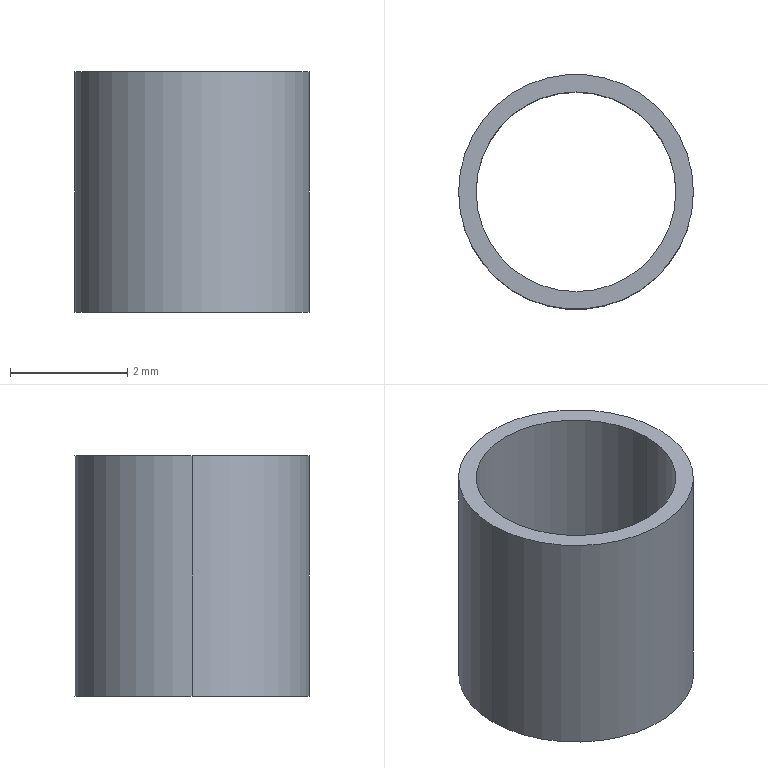Part | STEP file | Height-limit steel tube | 1 solid | 6 faces | box 4 x 4 x 4.1 mm | volume 14.297 mm3 | cylinder 4 | plane 2 | commonest cylinder face diameters 3.4 x2 4 x2
STEP:
#1=CARTESIAN_POINT('',(0.,0.,0.));
#2=DIRECTION('',(0.,0.,1.));
#3=DIRECTION('',(1.,0.,0.));
#4=AXIS2_PLACEMENT_3D('',#1,#2,#3);
#5=CARTESIAN_POINT('',(-1.7,0.,4.1));
#6=VERTEX_POINT('',#5);
#7=CARTESIAN_POINT('',(-1.7,0.,0.));
#8=VERTEX_POINT('',#7);
#9=CARTESIAN_POINT('',(-1.7,0.,4.1));
#10=DIRECTION('',(0.,0.,-1.));
#11=VECTOR('',#10,1.);
#12=LINE('',#9,#11);
#13=CARTESIAN_POINT('',(0.,0.,4.1));
#14=DIRECTION('',(0.,0.,-1.));
#15=DIRECTION('',(-1.,0.,0.));
#16=AXIS2_PLACEMENT_3D('',#13,#14,#15);
#17=CYLINDRICAL_SURFACE('',#16,1.7);
#18=CARTESIAN_POINT('',(6.283,0.));
#19=DIRECTION('',(0.,1.));
#20=VECTOR('',#19,1.);
#21=LINE('',#18,#20);
#22=(GEOMETRIC_REPRESENTATION_CONTEXT(2)PARAMETRIC_REPRESENTATION_CONTEXT()REPRESENTATION_CONTEXT('',''));
#23=DEFINITIONAL_REPRESENTATION('',(#21),#22);
#24=PCURVE('',#17,#23);
#25=CARTESIAN_POINT('',(0.,0.,4.1));
#26=DIRECTION('',(0.,0.,-1.));
#27=DIRECTION('',(-1.,0.,0.));
#28=AXIS2_PLACEMENT_3D('',#25,#26,#27);
#29=CYLINDRICAL_SURFACE('',#28,1.7);
#30=CARTESIAN_POINT('',(0.,0.));
#31=DIRECTION('',(0.,1.));
#32=VECTOR('',#31,1.);
#33=LINE('',#30,#32);
#34=(GEOMETRIC_REPRESENTATION_CONTEXT(2)PARAMETRIC_REPRESENTATION_CONTEXT()REPRESENTATION_CONTEXT('',''));
#35=DEFINITIONAL_REPRESENTATION('',(#33),#34);
#36=PCURVE('',#29,#35);
#37=SURFACE_CURVE('',#12,(#24,#36),.PCURVE_S1.);
#38=EDGE_CURVE('',#6,#8,#37,.T.);
#39=ORIENTED_EDGE('',*,*,#38,.T.);
#40=CARTESIAN_POINT('',(1.7,0.,0.));
#41=VERTEX_POINT('',#40);
#42=CARTESIAN_POINT('',(0.,0.,0.));
#43=DIRECTION('',(0.,0.,1.));
#44=DIRECTION('',(1.,0.,0.));
#45=AXIS2_PLACEMENT_3D('',#42,#43,#44);
#46=CIRCLE('',#45,1.7);
#47=CARTESIAN_POINT('',(9.425,4.1));
#48=DIRECTION('',(-1.,0.));
#49=VECTOR('',#48,1.);
#50=LINE('',#47,#49);
#51=(GEOMETRIC_REPRESENTATION_CONTEXT(2)PARAMETRIC_REPRESENTATION_CONTEXT()REPRESENTATION_CONTEXT('',''));
#52=DEFINITIONAL_REPRESENTATION('',(#50),#51);
#53=PCURVE('',#17,#52);
#54=CARTESIAN_POINT('',(0.,0.,0.));
#55=DIRECTION('',(0.,0.,1.));
#56=DIRECTION('',(1.,0.,0.));
#57=AXIS2_PLACEMENT_3D('',#54,#55,#56);
#58=PLANE('',#57);
#59=CARTESIAN_POINT('',(0.,0.));
#60=DIRECTION('',(1.,0.));
#61=AXIS2_PLACEMENT_2D('',#59,#60);
#62=CIRCLE('',#61,1.7);
#63=(GEOMETRIC_REPRESENTATION_CONTEXT(2)PARAMETRIC_REPRESENTATION_CONTEXT()REPRESENTATION_CONTEXT('',''));
#64=DEFINITIONAL_REPRESENTATION('',(#62),#63);
#65=PCURVE('',#58,#64);
#66=SURFACE_CURVE('',#46,(#53,#65),.PCURVE_S1.);
#67=EDGE_CURVE('',#8,#41,#66,.T.);
#68=ORIENTED_EDGE('',*,*,#67,.T.);
#69=CARTESIAN_POINT('',(1.7,0.,4.1));
#70=VERTEX_POINT('',#69);
#71=CARTESIAN_POINT('',(1.7,0.,4.1));
#72=DIRECTION('',(0.,0.,-1.));
#73=VECTOR('',#72,1.);
#74=LINE('',#71,#73);
#75=CARTESIAN_POINT('',(3.142,0.));
#76=DIRECTION('',(0.,1.));
#77=VECTOR('',#76,1.);
#78=LINE('',#75,#77);
#79=(GEOMETRIC_REPRESENTATION_CONTEXT(2)PARAMETRIC_REPRESENTATION_CONTEXT()REPRESENTATION_CONTEXT('',''));
#80=DEFINITIONAL_REPRESENTATION('',(#78),#79);
#81=PCURVE('',#17,#80);
#82=CARTESIAN_POINT('',(3.142,0.));
#83=DIRECTION('',(0.,1.));
#84=VECTOR('',#83,1.);
#85=LINE('',#82,#84);
#86=(GEOMETRIC_REPRESENTATION_CONTEXT(2)PARAMETRIC_REPRESENTATION_CONTEXT()REPRESENTATION_CONTEXT('',''));
#87=DEFINITIONAL_REPRESENTATION('',(#85),#86);
#88=PCURVE('',#29,#87);
#89=SURFACE_CURVE('',#74,(#81,#88),.PCURVE_S1.);
#90=EDGE_CURVE('',#70,#41,#89,.T.);
#91=ORIENTED_EDGE('',*,*,#90,.F.);
#92=CARTESIAN_POINT('',(0.,0.,4.1));
#93=DIRECTION('',(0.,0.,1.));
#94=DIRECTION('',(1.,0.,0.));
#95=AXIS2_PLACEMENT_3D('',#92,#93,#94);
#96=CIRCLE('',#95,1.7);
#97=CARTESIAN_POINT('',(9.425,0.));
#98=DIRECTION('',(-1.,0.));
#99=VECTOR('',#98,1.);
#100=LINE('',#97,#99);
#101=(GEOMETRIC_REPRESENTATION_CONTEXT(2)PARAMETRIC_REPRESENTATION_CONTEXT()REPRESENTATION_CONTEXT('',''));
#102=DEFINITIONAL_REPRESENTATION('',(#100),#101);
#103=PCURVE('',#17,#102);
#104=CARTESIAN_POINT('',(0.,0.,4.1));
#105=DIRECTION('',(0.,0.,1.));
#106=DIRECTION('',(1.,0.,0.));
#107=AXIS2_PLACEMENT_3D('',#104,#105,#106);
#108=PLANE('',#107);
#109=CARTESIAN_POINT('',(0.,0.));
#110=DIRECTION('',(1.,0.));
#111=AXIS2_PLACEMENT_2D('',#109,#110);
#112=CIRCLE('',#111,1.7);
#113=(GEOMETRIC_REPRESENTATION_CONTEXT(2)PARAMETRIC_REPRESENTATION_CONTEXT()REPRESENTATION_CONTEXT('',''));
#114=DEFINITIONAL_REPRESENTATION('',(#112),#113);
#115=PCURVE('',#108,#114);
#116=SURFACE_CURVE('',#96,(#103,#115),.PCURVE_S1.);
#117=EDGE_CURVE('',#6,#70,#116,.T.);
#118=ORIENTED_EDGE('',*,*,#117,.F.);
#119=EDGE_LOOP('',(#39,#68,#91,#118));
#120=FACE_BOUND('',#119,.F.);
#121=ADVANCED_FACE('',(#120),#17,.F.);
#122=CARTESIAN_POINT('',(2.,0.,4.1));
#123=VERTEX_POINT('',#122);
#124=CARTESIAN_POINT('',(-2.,0.,4.1));
#125=VERTEX_POINT('',#124);
#126=CARTESIAN_POINT('',(0.,0.,4.1));
#127=DIRECTION('',(0.,0.,1.));
#128=DIRECTION('',(1.,0.,0.));
#129=AXIS2_PLACEMENT_3D('',#126,#127,#128);
#130=CIRCLE('',#129,2.);
#131=CARTESIAN_POINT('',(0.,0.,4.1));
#132=DIRECTION('',(0.,0.,-1.));
#133=DIRECTION('',(-1.,0.,0.));
#134=AXIS2_PLACEMENT_3D('',#131,#132,#133);
#135=CYLINDRICAL_SURFACE('',#134,2.);
#136=CARTESIAN_POINT('',(3.142,0.));
#137=DIRECTION('',(-1.,0.));
#138=VECTOR('',#137,1.);
#139=LINE('',#136,#138);
#140=(GEOMETRIC_REPRESENTATION_CONTEXT(2)PARAMETRIC_REPRESENTATION_CONTEXT()REPRESENTATION_CONTEXT('',''));
#141=DEFINITIONAL_REPRESENTATION('',(#139),#140);
#142=PCURVE('',#135,#141);
#143=CARTESIAN_POINT('',(0.,0.));
#144=DIRECTION('',(1.,0.));
#145=AXIS2_PLACEMENT_2D('',#143,#144);
#146=CIRCLE('',#145,2.);
#147=(GEOMETRIC_REPRESENTATION_CONTEXT(2)PARAMETRIC_REPRESENTATION_CONTEXT()REPRESENTATION_CONTEXT('',''));
#148=DEFINITIONAL_REPRESENTATION('',(#146),#147);
#149=PCURVE('',#108,#148);
#150=SURFACE_CURVE('',#130,(#142,#149),.PCURVE_S1.);
#151=EDGE_CURVE('',#123,#125,#150,.T.);
#152=ORIENTED_EDGE('',*,*,#151,.F.);
#153=CARTESIAN_POINT('',(2.,0.,0.));
#154=VERTEX_POINT('',#153);
#155=CARTESIAN_POINT('',(2.,0.,4.1));
#156=DIRECTION('',(0.,0.,-1.));
#157=VECTOR('',#156,1.);
#158=LINE('',#155,#157);
#159=CARTESIAN_POINT('',(3.142,0.));
#160=DIRECTION('',(0.,1.));
#161=VECTOR('',#160,1.);
#162=LINE('',#159,#161);
#163=(GEOMETRIC_REPRESENTATION_CONTEXT(2)PARAMETRIC_REPRESENTATION_CONTEXT()REPRESENTATION_CONTEXT('',''));
#164=DEFINITIONAL_REPRESENTATION('',(#162),#163);
#165=PCURVE('',#135,#164);
#166=CARTESIAN_POINT('',(0.,0.,4.1));
#167=DIRECTION('',(0.,0.,-1.));
#168=DIRECTION('',(-1.,0.,0.));
#169=AXIS2_PLACEMENT_3D('',#166,#167,#168);
#170=CYLINDRICAL_SURFACE('',#169,2.);
#171=CARTESIAN_POINT('',(3.142,0.));
#172=DIRECTION('',(0.,1.));
#173=VECTOR('',#172,1.);
#174=LINE('',#171,#173);
#175=(GEOMETRIC_REPRESENTATION_CONTEXT(2)PARAMETRIC_REPRESENTATION_CONTEXT()REPRESENTATION_CONTEXT('',''));
#176=DEFINITIONAL_REPRESENTATION('',(#174),#175);
#177=PCURVE('',#170,#176);
#178=SURFACE_CURVE('',#158,(#165,#177),.PCURVE_S1.);
#179=EDGE_CURVE('',#123,#154,#178,.T.);
#180=ORIENTED_EDGE('',*,*,#179,.T.);
#181=CARTESIAN_POINT('',(-2.,0.,0.));
#182=VERTEX_POINT('',#181);
#183=CARTESIAN_POINT('',(0.,0.,0.));
#184=DIRECTION('',(0.,0.,1.));
#185=DIRECTION('',(1.,0.,0.));
#186=AXIS2_PLACEMENT_3D('',#183,#184,#185);
#187=CIRCLE('',#186,2.);
#188=CARTESIAN_POINT('',(3.142,4.1));
#189=DIRECTION('',(-1.,0.));
#190=VECTOR('',#189,1.);
#191=LINE('',#188,#190);
#192=(GEOMETRIC_REPRESENTATION_CONTEXT(2)PARAMETRIC_REPRESENTATION_CONTEXT()REPRESENTATION_CONTEXT('',''));
#193=DEFINITIONAL_REPRESENTATION('',(#191),#192);
#194=PCURVE('',#135,#193);
#195=CARTESIAN_POINT('',(0.,0.));
#196=DIRECTION('',(1.,0.));
#197=AXIS2_PLACEMENT_2D('',#195,#196);
#198=CIRCLE('',#197,2.);
#199=(GEOMETRIC_REPRESENTATION_CONTEXT(2)PARAMETRIC_REPRESENTATION_CONTEXT()REPRESENTATION_CONTEXT('',''));
#200=DEFINITIONAL_REPRESENTATION('',(#198),#199);
#201=PCURVE('',#58,#200);
#202=SURFACE_CURVE('',#187,(#194,#201),.PCURVE_S1.);
#203=EDGE_CURVE('',#154,#182,#202,.T.);
#204=ORIENTED_EDGE('',*,*,#203,.T.);
#205=CARTESIAN_POINT('',(-2.,0.,4.1));
#206=DIRECTION('',(0.,0.,-1.));
#207=VECTOR('',#206,1.);
#208=LINE('',#205,#207);
#209=CARTESIAN_POINT('',(0.,0.));
#210=DIRECTION('',(0.,1.));
#211=VECTOR('',#210,1.);
#212=LINE('',#209,#211);
#213=(GEOMETRIC_REPRESENTATION_CONTEXT(2)PARAMETRIC_REPRESENTATION_CONTEXT()REPRESENTATION_CONTEXT('',''));
#214=DEFINITIONAL_REPRESENTATION('',(#212),#213);
#215=PCURVE('',#135,#214);
#216=CARTESIAN_POINT('',(6.283,0.));
#217=DIRECTION('',(0.,1.));
#218=VECTOR('',#217,1.);
#219=LINE('',#216,#218);
#220=(GEOMETRIC_REPRESENTATION_CONTEXT(2)PARAMETRIC_REPRESENTATION_CONTEXT()REPRESENTATION_CONTEXT('',''));
#221=DEFINITIONAL_REPRESENTATION('',(#219),#220);
#222=PCURVE('',#170,#221);
#223=SURFACE_CURVE('',#208,(#215,#222),.PCURVE_S1.);
#224=EDGE_CURVE('',#125,#182,#223,.T.);
#225=ORIENTED_EDGE('',*,*,#224,.F.);
#226=EDGE_LOOP('',(#152,#180,#204,#225));
#227=FACE_BOUND('',#226,.T.);
#228=ADVANCED_FACE('',(#227),#135,.T.);
#229=CARTESIAN_POINT('',(0.,0.,4.1));
#230=DIRECTION('',(0.,0.,1.));
#231=DIRECTION('',(1.,0.,0.));
#232=AXIS2_PLACEMENT_3D('',#229,#230,#231);
#233=CIRCLE('',#232,2.);
#234=CARTESIAN_POINT('',(0.,0.));
#235=DIRECTION('',(1.,0.));
#236=AXIS2_PLACEMENT_2D('',#234,#235);
#237=CIRCLE('',#236,2.);
#238=(GEOMETRIC_REPRESENTATION_CONTEXT(2)PARAMETRIC_REPRESENTATION_CONTEXT()REPRESENTATION_CONTEXT('',''));
#239=DEFINITIONAL_REPRESENTATION('',(#237),#238);
#240=PCURVE('',#108,#239);
#241=CARTESIAN_POINT('',(9.425,0.));
#242=DIRECTION('',(-1.,0.));
#243=VECTOR('',#242,1.);
#244=LINE('',#241,#243);
#245=(GEOMETRIC_REPRESENTATION_CONTEXT(2)PARAMETRIC_REPRESENTATION_CONTEXT()REPRESENTATION_CONTEXT('',''));
#246=DEFINITIONAL_REPRESENTATION('',(#244),#245);
#247=PCURVE('',#170,#246);
#248=SURFACE_CURVE('',#233,(#240,#247),.PCURVE_S1.);
#249=EDGE_CURVE('',#125,#123,#248,.T.);
#250=ORIENTED_EDGE('',*,*,#249,.T.);
#251=ORIENTED_EDGE('',*,*,#151,.T.);
#252=EDGE_LOOP('',(#250,#251));
#253=FACE_BOUND('',#252,.T.);
#254=ORIENTED_EDGE('',*,*,#117,.F.);
#255=CARTESIAN_POINT('',(0.,0.,4.1));
#256=DIRECTION('',(0.,0.,1.));
#257=DIRECTION('',(1.,0.,0.));
#258=AXIS2_PLACEMENT_3D('',#255,#256,#257);
#259=CIRCLE('',#258,1.7);
#260=CARTESIAN_POINT('',(0.,0.));
#261=DIRECTION('',(1.,0.));
#262=AXIS2_PLACEMENT_2D('',#260,#261);
#263=CIRCLE('',#262,1.7);
#264=(GEOMETRIC_REPRESENTATION_CONTEXT(2)PARAMETRIC_REPRESENTATION_CONTEXT()REPRESENTATION_CONTEXT('',''));
#265=DEFINITIONAL_REPRESENTATION('',(#263),#264);
#266=PCURVE('',#108,#265);
#267=CARTESIAN_POINT('',(3.142,0.));
#268=DIRECTION('',(-1.,0.));
#269=VECTOR('',#268,1.);
#270=LINE('',#267,#269);
#271=(GEOMETRIC_REPRESENTATION_CONTEXT(2)PARAMETRIC_REPRESENTATION_CONTEXT()REPRESENTATION_CONTEXT('',''));
#272=DEFINITIONAL_REPRESENTATION('',(#270),#271);
#273=PCURVE('',#29,#272);
#274=SURFACE_CURVE('',#259,(#266,#273),.PCURVE_S1.);
#275=EDGE_CURVE('',#70,#6,#274,.T.);
#276=ORIENTED_EDGE('',*,*,#275,.F.);
#277=EDGE_LOOP('',(#254,#276));
#278=FACE_BOUND('',#277,.T.);
#279=ADVANCED_FACE('',(#253,#278),#108,.T.);
#280=CARTESIAN_POINT('',(0.,0.,0.));
#281=DIRECTION('',(0.,0.,1.));
#282=DIRECTION('',(1.,0.,0.));
#283=AXIS2_PLACEMENT_3D('',#280,#281,#282);
#284=CIRCLE('',#283,2.);
#285=CARTESIAN_POINT('',(0.,0.));
#286=DIRECTION('',(1.,0.));
#287=AXIS2_PLACEMENT_2D('',#285,#286);
#288=CIRCLE('',#287,2.);
#289=(GEOMETRIC_REPRESENTATION_CONTEXT(2)PARAMETRIC_REPRESENTATION_CONTEXT()REPRESENTATION_CONTEXT('',''));
#290=DEFINITIONAL_REPRESENTATION('',(#288),#289);
#291=PCURVE('',#58,#290);
#292=CARTESIAN_POINT('',(9.425,4.1));
#293=DIRECTION('',(-1.,0.));
#294=VECTOR('',#293,1.);
#295=LINE('',#292,#294);
#296=(GEOMETRIC_REPRESENTATION_CONTEXT(2)PARAMETRIC_REPRESENTATION_CONTEXT()REPRESENTATION_CONTEXT('',''));
#297=DEFINITIONAL_REPRESENTATION('',(#295),#296);
#298=PCURVE('',#170,#297);
#299=SURFACE_CURVE('',#284,(#291,#298),.PCURVE_S1.);
#300=EDGE_CURVE('',#182,#154,#299,.T.);
#301=ORIENTED_EDGE('',*,*,#300,.F.);
#302=ORIENTED_EDGE('',*,*,#203,.F.);
#303=EDGE_LOOP('',(#301,#302));
#304=FACE_BOUND('',#303,.T.);
#305=ORIENTED_EDGE('',*,*,#67,.T.);
#306=CARTESIAN_POINT('',(0.,0.,0.));
#307=DIRECTION('',(0.,0.,1.));
#308=DIRECTION('',(1.,0.,0.));
#309=AXIS2_PLACEMENT_3D('',#306,#307,#308);
#310=CIRCLE('',#309,1.7);
#311=CARTESIAN_POINT('',(0.,0.));
#312=DIRECTION('',(1.,0.));
#313=AXIS2_PLACEMENT_2D('',#311,#312);
#314=CIRCLE('',#313,1.7);
#315=(GEOMETRIC_REPRESENTATION_CONTEXT(2)PARAMETRIC_REPRESENTATION_CONTEXT()REPRESENTATION_CONTEXT('',''));
#316=DEFINITIONAL_REPRESENTATION('',(#314),#315);
#317=PCURVE('',#58,#316);
#318=CARTESIAN_POINT('',(3.142,4.1));
#319=DIRECTION('',(-1.,0.));
#320=VECTOR('',#319,1.);
#321=LINE('',#318,#320);
#322=(GEOMETRIC_REPRESENTATION_CONTEXT(2)PARAMETRIC_REPRESENTATION_CONTEXT()REPRESENTATION_CONTEXT('',''));
#323=DEFINITIONAL_REPRESENTATION('',(#321),#322);
#324=PCURVE('',#29,#323);
#325=SURFACE_CURVE('',#310,(#317,#324),.PCURVE_S1.);
#326=EDGE_CURVE('',#41,#8,#325,.T.);
#327=ORIENTED_EDGE('',*,*,#326,.T.);
#328=EDGE_LOOP('',(#305,#327));
#329=FACE_BOUND('',#328,.T.);
#330=ADVANCED_FACE('',(#304,#329),#58,.F.);
#331=ORIENTED_EDGE('',*,*,#179,.F.);
#332=ORIENTED_EDGE('',*,*,#249,.F.);
#333=ORIENTED_EDGE('',*,*,#224,.T.);
#334=ORIENTED_EDGE('',*,*,#300,.T.);
#335=EDGE_LOOP('',(#331,#332,#333,#334));
#336=FACE_BOUND('',#335,.T.);
#337=ADVANCED_FACE('',(#336),#170,.T.);
#338=ORIENTED_EDGE('',*,*,#326,.T.);
#339=ORIENTED_EDGE('',*,*,#38,.F.);
#340=ORIENTED_EDGE('',*,*,#275,.F.);
#341=ORIENTED_EDGE('',*,*,#90,.T.);
#342=EDGE_LOOP('',(#338,#339,#340,#341));
#343=FACE_BOUND('',#342,.F.);
#344=ADVANCED_FACE('',(#343),#29,.F.);
#345=CLOSED_SHELL('',(#121,#228,#279,#330,#337,#344));
#346=MANIFOLD_SOLID_BREP('',#345);
#347=(LENGTH_UNIT()NAMED_UNIT(*)SI_UNIT(.MILLI.,.METRE.));
#348=UNCERTAINTY_MEASURE_WITH_UNIT(LENGTH_MEASURE(0.0000001),#347,'','');
#349=(NAMED_UNIT(*)PLANE_ANGLE_UNIT()SI_UNIT($,.RADIAN.));
#350=(NAMED_UNIT(*)SI_UNIT($,.STERADIAN.)SOLID_ANGLE_UNIT());
#351=(GEOMETRIC_REPRESENTATION_CONTEXT(3)GLOBAL_UNCERTAINTY_ASSIGNED_CONTEXT((#348))GLOBAL_UNIT_ASSIGNED_CONTEXT((#347,#349,#350))REPRESENTATION_CONTEXT('',''));
#352=ADVANCED_BREP_SHAPE_REPRESENTATION('',(#4,#346),#351);